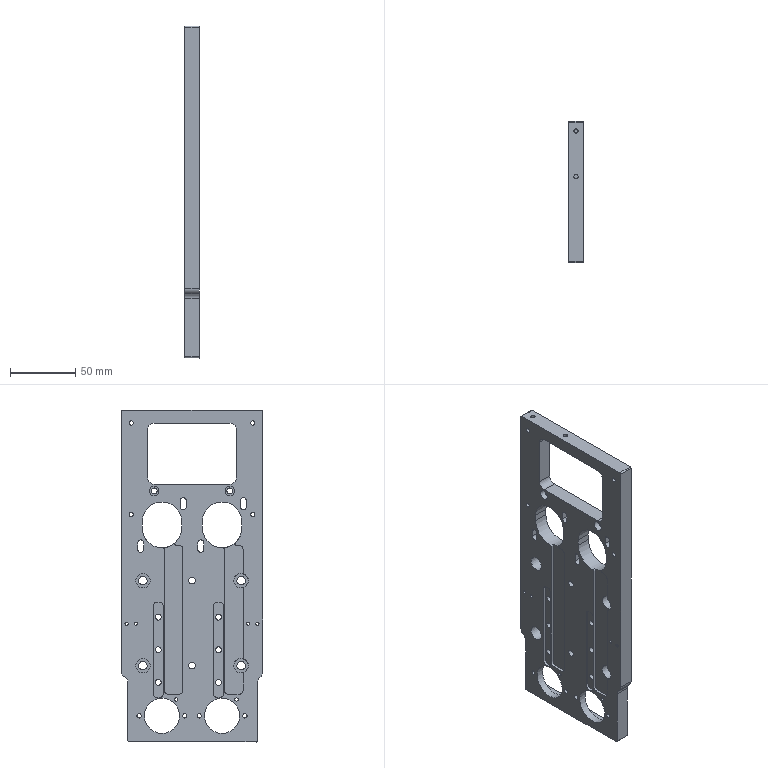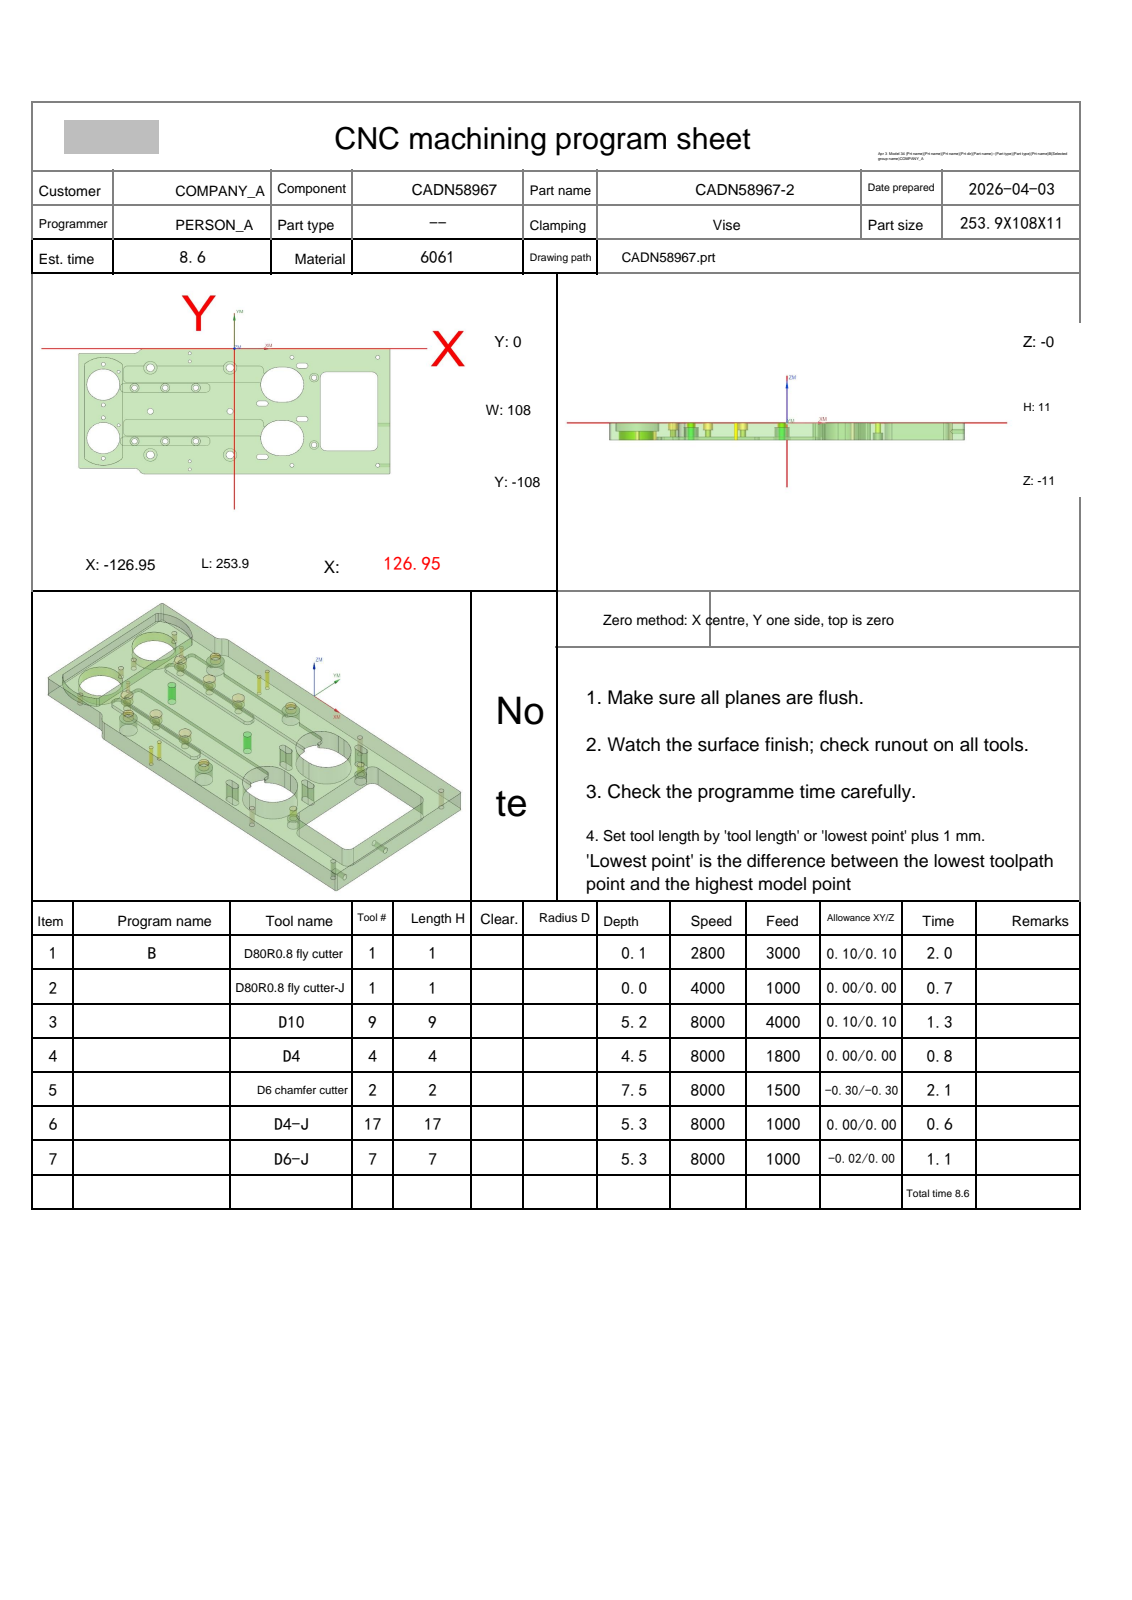NC program | NX | posted by the shop | part box 11 x 108 x 253.9 mm
Lines 1506 to 2432 of 3878:
N6 T17 M06
(D4-J  D=4. R=0. H=17 ce=0.00 di=0.00)
G00 G90 G54 X-118.616 Y-13.414 M03 S8000
G43 H17 Z20.
M08
Z.159
G01 X-118.62 Y-13.41 Z.098 F1000.
X-118.631 Y-13.401 Z.044
X-118.649 Y-13.386 Z-.005
X-118.673 Y-13.368 Z-.049
X-118.702 Y-13.347 Z-.087
X-118.736 Y-13.326 Z-.12
X-118.775 Y-13.305 Z-.148
X-118.817 Y-13.286 Z-.172
X-118.863 Y-13.269 Z-.192
X-118.911 Y-13.258 Z-.208
X-118.962 Y-13.252 Z-.221
X-119.014 Y-13.253 Z-.23
X-119.066 Y-13.262 Z-.236
X-119.12 Y-13.282 Z-.24
X-119.173 Y-13.312 Z-.241
G03 X-120.45 Y-14.267 I12.223 J-17.688
G01 Y-15.771
X-120.437 Y-15.822
X-120.399 Y-15.843 Z-.242
X-120.341 Y-15.837 Z-.244
X-120.265 Y-15.806 Z-.247
X-120.177 Y-15.754 Z-.251
X-120.078 Y-15.682 Z-.256
X-119.974 Y-15.594 Z-.262
X-119.868 Y-15.493 Z-.27
X-119.763 Y-15.38 Z-.279
X-119.546 Y-15.098 Z-.304
X-119.359 Y-14.785 Z-.335
X-119.21 Y-14.452 Z-.368
X-119.103 Y-14.11 Z-.401
X-119.071 Y-13.958 Z-.415
X-119.048 Y-13.812 Z-.429
X-119.035 Y-13.675 Z-.441
X-119.032 Y-13.552 Z-.453
X-119.039 Y-13.447 Z-.462
X-119.057 Y-13.367 Z-.471
X-119.085 Y-13.314 Z-.477
X-119.123 Y-13.294 Z-.48
X-119.173 Y-13.312 Z-.482
G03 X-120.45 Y-14.267 I12.223 J-17.688
G01 Y-15.771
X-120.437 Y-15.822
X-120.399 Y-15.844 Z-.483
X-120.341 Y-15.838 Z-.485
X-120.265 Y-15.808 Z-.488
X-120.177 Y-15.756 Z-.493
X-120.079 Y-15.686 Z-.498
X-119.974 Y-15.599 Z-.504
X-119.868 Y-15.498 Z-.512
X-119.763 Y-15.386 Z-.521
X-119.546 Y-15.104 Z-.546
X-119.359 Y-14.791 Z-.577
X-119.21 Y-14.457 Z-.61
X-119.103 Y-14.113 Z-.643
X-119.071 Y-13.961 Z-.657
X-119.048 Y-13.814 Z-.67
X-119.035 Y-13.676 Z-.683
X-119.032 Y-13.553 Z-.694
X-119.039 Y-13.448 Z-.704
X-119.057 Y-13.367 Z-.712
X-119.085 Y-13.314 Z-.718
X-119.123 Y-13.295 Z-.721
X-119.173 Y-13.312 Z-.723
G03 X-120.45 Y-14.267 I12.223 J-17.688
G01 Y-15.771
X-120.437 Y-15.823
X-120.399 Y-15.844 Z-.724
X-120.341 Y-15.839 Z-.727
X-120.265 Y-15.81 Z-.73
X-120.177 Y-15.759 Z-.734
X-120.079 Y-15.689 Z-.739
X-119.975 Y-15.603 Z-.746
X-119.868 Y-15.503 Z-.754
X-119.764 Y-15.392 Z-.763
X-119.587 Y-15.17 Z-.783
X-119.43 Y-14.925 Z-.806
X-119.295 Y-14.664 Z-.832
X-119.185 Y-14.393 Z-.858
X-119.104 Y-14.117 Z-.884
X-119.071 Y-13.964 Z-.898
X-119.048 Y-13.816 Z-.911
X-119.035 Y-13.678 Z-.924
X-119.032 Y-13.554 Z-.935
X-119.039 Y-13.449 Z-.945
X-119.057 Y-13.368 Z-.953
X-119.085 Y-13.315 Z-.959
X-119.123 Y-13.295 Z-.962
X-119.173 Y-13.312 Z-.964
G03 X-120.45 Y-14.267 I12.223 J-17.688
G01 Y-15.771
X-120.437 Y-15.823
X-120.399 Y-15.845 Z-.965
X-120.341 Y-15.841 Z-.968
X-120.265 Y-15.812 Z-.971
X-120.177 Y-15.762 Z-.975
X-120.079 Y-15.693 Z-.981
X-119.975 Y-15.608 Z-.988
X-119.869 Y-15.508 Z-.996
X-119.764 Y-15.397 Z-1.005
X-119.588 Y-15.176 Z-1.025
X-119.43 Y-14.931 Z-1.048
X-119.296 Y-14.67 Z-1.074
X-119.186 Y-14.397 Z-1.1
X-119.104 Y-14.12 Z-1.126
X-119.071 Y-13.966 Z-1.14
X-119.048 Y-13.818 Z-1.153
X-119.035 Y-13.679 Z-1.165
X-119.032 Y-13.555 Z-1.176
X-119.039 Y-13.45 Z-1.186
X-119.057 Y-13.368 Z-1.194
X-119.085 Y-13.315 Z-1.199
X-119.123 Y-13.295 Z-1.203
X-119.173 Y-13.312 Z-1.205
G03 X-120.45 Y-14.267 I12.223 J-17.688
G01 Y-15.771
X-120.437 Y-15.823
X-120.399 Y-15.846 Z-1.206
X-120.341 Y-15.842 Z-1.209
X-120.266 Y-15.814 Z-1.212
X-120.177 Y-15.765 Z-1.217
X-120.079 Y-15.697 Z-1.223
X-119.975 Y-15.612 Z-1.229
X-119.869 Y-15.514 Z-1.238
X-119.765 Y-15.403 Z-1.247
X-119.588 Y-15.182 Z-1.267
X-119.431 Y-14.937 Z-1.29
X-119.296 Y-14.675 Z-1.315
X-119.186 Y-14.401 Z-1.342
X-119.104 Y-14.123 Z-1.367
X-119.072 Y-13.969 Z-1.381
X-119.049 Y-13.82 Z-1.394
X-119.035 Y-13.681 Z-1.406
X-119.032 Y-13.556 Z-1.417
X-119.039 Y-13.451 Z-1.427
X-119.057 Y-13.369 Z-1.435
X-119.085 Y-13.315 Z-1.44
X-119.123 Y-13.295 Z-1.444
X-119.173 Y-13.312 Z-1.445
G03 X-120.45 Y-14.267 I12.223 J-17.688
G01 Y-15.771
X-120.437 Y-15.823 Z-1.446
X-120.399 Y-15.846 Z-1.447
X-120.341 Y-15.843 Z-1.45
X-120.266 Y-15.816 Z-1.454
X-120.178 Y-15.768 Z-1.458
X-120.08 Y-15.701 Z-1.464
X-119.976 Y-15.617 Z-1.471
X-119.87 Y-15.519 Z-1.48
X-119.765 Y-15.409 Z-1.489
X-119.589 Y-15.188 Z-1.509
X-119.432 Y-14.943 Z-1.532
X-119.297 Y-14.68 Z-1.557
X-119.187 Y-14.406 Z-1.583
X-119.105 Y-14.126 Z-1.609
X-119.072 Y-13.972 Z-1.623
X-119.049 Y-13.822 Z-1.635
X-119.036 Y-13.683 Z-1.648
X-119.033 Y-13.557 Z-1.658
X-119.039 Y-13.451 Z-1.668
X-119.057 Y-13.369 Z-1.676
X-119.085 Y-13.315 Z-1.681
X-119.123 Y-13.295 Z-1.685
X-119.173 Y-13.312 Z-1.686
G03 X-120.45 Y-14.267 I12.223 J-17.688
G01 Y-15.771
X-120.437 Y-15.823 Z-1.687
X-120.399 Y-15.847 Z-1.688
X-120.341 Y-15.844 Z-1.691
X-120.266 Y-15.818 Z-1.695
X-120.178 Y-15.771 Z-1.7
X-120.08 Y-15.704 Z-1.706
X-119.977 Y-15.621 Z-1.713
X-119.871 Y-15.524 Z-1.722
X-119.766 Y-15.415 Z-1.731
X-119.59 Y-15.194 Z-1.751
X-119.433 Y-14.949 Z-1.774
X-119.298 Y-14.685 Z-1.799
X-119.187 Y-14.41 Z-1.825
X-119.105 Y-14.13 Z-1.85
X-119.072 Y-13.975 Z-1.864
X-119.049 Y-13.825 Z-1.877
X-119.036 Y-13.684 Z-1.889
X-119.033 Y-13.559 Z-1.9
X-119.04 Y-13.452 Z-1.909
X-119.057 Y-13.369 Z-1.917
X-119.085 Y-13.316 Z-1.922
X-119.123 Y-13.295 Z-1.926
X-119.173 Y-13.312 Z-1.927
G03 X-120.45 Y-14.267 I12.223 J-17.688
G01 Y-15.771
X-120.437 Y-15.823 Z-1.928
X-120.399 Y-15.847 Z-1.93
X-120.341 Y-15.845 Z-1.932
X-120.267 Y-15.82 Z-1.936
X-120.179 Y-15.774 Z-1.941
X-120.081 Y-15.708 Z-1.948
X-119.978 Y-15.626 Z-1.955
X-119.872 Y-15.529 Z-1.964
X-119.767 Y-15.421 Z-1.973
X-119.591 Y-15.201 Z-1.994
X-119.434 Y-14.955 Z-2.017
X-119.299 Y-14.691 Z-2.041
X-119.188 Y-14.415 Z-2.067
X-119.106 Y-14.133 Z-2.092
X-119.073 Y-13.977 Z-2.105
X-119.05 Y-13.827 Z-2.118
X-119.036 Y-13.686 Z-2.13
X-119.033 Y-13.56 Z-2.141
X-119.04 Y-13.453 Z-2.15
X-119.057 Y-13.37 Z-2.158
X-119.085 Y-13.316 Z-2.163
X-119.123 Y-13.295 Z-2.167
X-119.173 Y-13.312 Z-2.168
G03 X-120.45 Y-14.267 I12.223 J-17.688
G01 Y-15.771
X-120.437 Y-15.824 Z-2.169
X-120.399 Y-15.848 Z-2.171
X-120.342 Y-15.847 Z-2.173
X-120.267 Y-15.822 Z-2.178
X-120.179 Y-15.776 Z-2.183
X-120.082 Y-15.712 Z-2.189
X-119.979 Y-15.631 Z-2.197
X-119.873 Y-15.535 Z-2.206
X-119.769 Y-15.427 Z-2.215
X-119.593 Y-15.207 Z-2.236
X-119.435 Y-14.961 Z-2.259
X-119.3 Y-14.696 Z-2.284
X-119.189 Y-14.419 Z-2.309
X-119.106 Y-14.136 Z-2.334
X-119.073 Y-13.98 Z-2.347
X-119.05 Y-13.829 Z-2.36
X-119.037 Y-13.688 Z-2.371
X-119.033 Y-13.561 Z-2.382
X-119.04 Y-13.454 Z-2.391
X-119.057 Y-13.37 Z-2.399
X-119.085 Y-13.316 Z-2.404
X-119.123 Y-13.295 Z-2.408
X-119.173 Y-13.312 Z-2.409
G03 X-120.45 Y-14.267 I12.223 J-17.688
G01 Y-15.771
X-120.437 Y-15.824 Z-2.41
X-120.4 Y-15.848 Z-2.412
X-120.342 Z-2.415
X-120.268 Y-15.824 Z-2.419
X-120.18 Y-15.779 Z-2.424
X-120.083 Y-15.716 Z-2.431
X-119.98 Y-15.635 Z-2.439
X-119.874 Y-15.54 Z-2.448
X-119.77 Y-15.432 Z-2.458
X-119.594 Y-15.213 Z-2.478
X-119.437 Y-14.967 Z-2.501
X-119.301 Y-14.701 Z-2.526
X-119.19 Y-14.423 Z-2.551
X-119.107 Y-14.14 Z-2.575
X-119.074 Y-13.983 Z-2.588
X-119.051 Y-13.831 Z-2.601
X-119.037 Y-13.689 Z-2.613
X-119.034 Y-13.562 Z-2.623
X-119.04 Y-13.454 Z-2.632
X-119.057 Y-13.371 Z-2.64
X-119.085 Y-13.316 Z-2.645
X-119.123 Y-13.295 Z-2.649
X-119.173 Y-13.312 Z-2.65
G03 X-120.45 Y-14.267 I12.223 J-17.688
G01 Y-15.771
X-120.437 Y-15.824 Z-2.651
X-120.4 Y-15.849 Z-2.653
X-120.342 Z-2.656
X-120.268 Y-15.826 Z-2.66
X-120.181 Y-15.782 Z-2.666
X-120.084 Y-15.719 Z-2.673
X-119.981 Y-15.64 Z-2.681
X-119.876 Y-15.545 Z-2.69
X-119.772 Y-15.438 Z-2.7
X-119.596 Y-15.219 Z-2.72
X-119.439 Y-14.973 Z-2.743
X-119.303 Y-14.707 Z-2.768
X-119.192 Y-14.428 Z-2.793
X-119.108 Y-14.143 Z-2.817
X-119.078 Y-14.001 Z-2.829
X-119.055 Y-13.863 Z-2.84
X-119.041 Y-13.732 Z-2.85
X-119.034 Y-13.612 Z-2.86
X-119.036 Y-13.507 Z-2.869
X-119.046 Y-13.419 Z-2.876
X-119.064 Y-13.352 Z-2.882
X-119.092 Y-13.309 Z-2.887
X-119.128 Y-13.295 Z-2.89
X-119.173 Y-13.312 Z-2.891
G03 X-120.45 Y-14.267 I12.223 J-17.688
G01 Y-15.771
X-120.437 Y-15.824 Z-2.892
X-120.4 Y-15.85 Z-2.894
X-120.343 Z-2.897
X-120.269 Y-15.828 Z-2.902
X-120.182 Y-15.785 Z-2.908
X-120.085 Y-15.723 Z-2.915
X-119.983 Y-15.644 Z-2.923
X-119.878 Y-15.55 Z-2.932
X-119.774 Y-15.444 Z-2.942
X-119.598 Y-15.225 Z-2.963
X-119.441 Y-14.979 Z-2.986
X-119.305 Y-14.712 Z-3.01
X-119.193 Y-14.432 Z-3.034
X-119.109 Y-14.146 Z-3.059
X-119.079 Y-14.004 Z-3.07
X-119.056 Y-13.865 Z-3.081
X-119.041 Y-13.734 Z-3.092
X-119.035 Y-13.614 Z-3.101
X-119.036 Y-13.508 Z-3.11
X-119.046 Y-13.419 Z-3.117
X-119.065 Y-13.352 Z-3.123
X-119.092 Y-13.309 Z-3.128
X-119.128 Y-13.295 Z-3.131
X-119.173 Y-13.312 Z-3.132
G03 X-120.45 Y-14.267 I12.223 J-17.688
G01 Y-15.771
X-120.437 Y-15.824 Z-3.133
X-120.4 Y-15.85 Z-3.135
X-120.343 Y-15.852 Z-3.138
X-120.27 Y-15.83 Z-3.143
X-120.183 Y-15.788 Z-3.149
X-120.087 Y-15.727 Z-3.156
X-119.984 Y-15.649 Z-3.165
X-119.88 Y-15.556 Z-3.174
X-119.776 Y-15.45 Z-3.184
X-119.6 Y-15.231 Z-3.205
X-119.443 Y-14.985 Z-3.228
X-119.307 Y-14.717 Z-3.252
X-119.195 Y-14.436 Z-3.276
X-119.111 Y-14.149 Z-3.3
X-119.08 Y-14.006 Z-3.312
X-119.057 Y-13.867 Z-3.323
X-119.042 Y-13.736 Z-3.333
X-119.035 Y-13.615 Z-3.343
X-119.037 Y-13.509 Z-3.351
X-119.046 Y-13.42 Z-3.358
X-119.065 Y-13.352 Z-3.364
X-119.092 Y-13.31 Z-3.369
X-119.128 Y-13.295 Z-3.372
X-119.173 Y-13.312 Z-3.373
G03 X-120.45 Y-14.267 I12.223 J-17.688
G01 Y-15.771
X-120.437 Y-15.824 Z-3.374
X-120.4 Y-15.851 Z-3.376
X-120.344 Y-15.853 Z-3.379
X-120.27 Y-15.832 Z-3.384
X-120.184 Y-15.791 Z-3.391
X-120.088 Y-15.73 Z-3.398
X-119.986 Y-15.653 Z-3.407
X-119.882 Y-15.561 Z-3.416
X-119.778 Y-15.455 Z-3.427
X-119.603 Y-15.237 Z-3.447
X-119.445 Y-14.99 Z-3.47
X-119.309 Y-14.722 Z-3.494
X-119.196 Y-14.44 Z-3.518
X-119.112 Y-14.152 Z-3.542
X-119.081 Y-14.009 Z-3.553
X-119.058 Y-13.87 Z-3.564
X-119.043 Y-13.738 Z-3.574
X-119.036 Y-13.616 Z-3.584
X-119.037 Y-13.509 Z-3.592
X-119.047 Y-13.42 Z-3.6
X-119.065 Y-13.353 Z-3.605
X-119.092 Y-13.31 Z-3.61
X-119.128 Y-13.295 Z-3.613
X-119.173 Y-13.312 Z-3.614
G03 X-120.45 Y-14.267 I12.223 J-17.688
G01 Y-15.771
X-120.437 Y-15.824
X-120.401 Y-15.851 Z-3.617
X-120.344 Y-15.854 Z-3.621
X-120.271 Y-15.834 Z-3.626
X-120.185 Y-15.793 Z-3.632
X-120.09 Y-15.734 Z-3.64
X-119.988 Y-15.657 Z-3.649
X-119.884 Y-15.566 Z-3.658
X-119.781 Y-15.461 Z-3.669
X-119.605 Y-15.243 Z-3.69
X-119.448 Y-14.996 Z-3.713
X-119.311 Y-14.727 Z-3.736
X-119.198 Y-14.445 Z-3.76
X-119.113 Y-14.156 Z-3.784
X-119.082 Y-14.012 Z-3.795
X-119.059 Y-13.872 Z-3.806
X-119.043 Y-13.739 Z-3.816
X-119.036 Y-13.618 Z-3.825
X-119.037 Y-13.51 Z-3.833
X-119.047 Y-13.421 Z-3.841
X-119.065 Y-13.353 Z-3.846
X-119.092 Y-13.31 Z-3.851
X-119.128 Y-13.295 Z-3.854
X-119.173 Y-13.312 Z-3.855
G03 X-120.45 Y-14.267 I12.223 J-17.688
G01 Y-15.771
X-120.437 Y-15.825
X-120.401 Y-15.852 Z-3.858
X-120.345 Y-15.855 Z-3.862
X-120.272 Y-15.836 Z-3.867
X-120.187 Y-15.796 Z-3.874
X-120.092 Y-15.737 Z-3.882
X-119.99 Y-15.662 Z-3.891
X-119.886 Y-15.571 Z-3.9
X-119.783 Y-15.466 Z-3.911
X-119.608 Y-15.249 Z-3.932
X-119.451 Y-15.002 Z-3.955
X-119.313 Y-14.732 Z-3.978
X-119.2 Y-14.449 Z-4.002
X-119.115 Y-14.159 Z-4.025
X-119.083 Y-14.014 Z-4.036
X-119.06 Y-13.874 Z-4.047
X-119.044 Y-13.741 Z-4.057
X-119.037 Y-13.619 Z-4.066
X-119.038 Y-13.511 Z-4.075
X-119.047 Y-13.422 Z-4.082
X-119.065 Y-13.353 Z-4.087
X-119.092 Y-13.31 Z-4.092
X-119.128 Y-13.295 Z-4.095
X-119.173 Y-13.312
G03 X-120.45 Y-14.267 I12.223 J-17.688
G01 Y-15.771
X-120.437 Y-15.825 Z-4.096
X-120.401 Y-15.852 Z-4.099
X-120.345 Y-15.856 Z-4.103
X-120.273 Y-15.838 Z-4.109
X-120.188 Y-15.799 Z-4.115
X-120.093 Y-15.741 Z-4.124
X-119.993 Y-15.666 Z-4.133
X-119.889 Y-15.576 Z-4.143
X-119.786 Y-15.472 Z-4.154
X-119.611 Y-15.255 Z-4.175
X-119.453 Y-15.007 Z-4.197
X-119.316 Y-14.737 Z-4.221
X-119.203 Y-14.453 Z-4.244
X-119.116 Y-14.162 Z-4.267
X-119.085 Y-14.017 Z-4.278
X-119.061 Y-13.876 Z-4.289
X-119.045 Y-13.743 Z-4.298
X-119.038 Y-13.62 Z-4.308
Y-13.512 Z-4.316
X-119.048 Y-13.422 Z-4.323
X-119.065 Y-13.354 Z-4.328
X-119.092 Y-13.31 Z-4.333
X-119.128 Y-13.295 Z-4.335
X-119.173 Y-13.312 Z-4.336
G03 X-120.45 Y-14.267 I12.223 J-17.688
G01 Y-15.771
X-120.435 Y-15.831 Z-4.338
X-120.394 Y-15.862 Z-4.342
X-120.331 Y-15.865 Z-4.348
X-120.25 Y-15.843 Z-4.356
X-120.155 Y-15.795 Z-4.366
X-120.051 Y-15.726 Z-4.377
X-119.941 Y-15.635 Z-4.389
X-119.83 Y-15.524 Z-4.402
X-119.658 Y-15.311 Z-4.423
X-119.498 Y-15.061 Z-4.446
X-119.356 Y-14.785 Z-4.468
X-119.235 Y-14.492 Z-4.49
X-119.141 Y-14.191 Z-4.512
X-119.105 Y-14.042 Z-4.522
X-119.078 Y-13.896 Z-4.532
X-119.059 Y-13.759 Z-4.542
X-119.048 Y-13.632 Z-4.55
X-119.046 Y-13.521 Z-4.558
X-119.052 Y-13.428 Z-4.564
X-119.068 Y-13.357 Z-4.57
X-119.093 Y-13.312 Z-4.574
X-119.128 Y-13.296 Z-4.576
X-119.173 Y-13.312 Z-4.577
G03 X-120.45 Y-14.267 I12.223 J-17.688
G01 Y-15.771
X-120.435 Y-15.831 Z-4.579
X-120.394 Y-15.862 Z-4.583
X-120.331 Y-15.865 Z-4.589
X-120.25 Y-15.843 Z-4.597
X-120.155 Y-15.795 Z-4.606
X-120.051 Y-15.726 Z-4.618
X-119.941 Y-15.635 Z-4.63
X-119.83 Y-15.524 Z-4.643
X-119.658 Y-15.311 Z-4.664
X-119.498 Y-15.061 Z-4.686
X-119.356 Y-14.785 Z-4.709
X-119.235 Y-14.492 Z-4.731
X-119.141 Y-14.191 Z-4.753
X-119.105 Y-14.042 Z-4.763
X-119.078 Y-13.896 Z-4.773
X-119.059 Y-13.759 Z-4.783
X-119.048 Y-13.632 Z-4.791
X-119.046 Y-13.521 Z-4.799
X-119.052 Y-13.428 Z-4.805
X-119.068 Y-13.357 Z-4.811
X-119.093 Y-13.312 Z-4.815
X-119.128 Y-13.296 Z-4.817
X-119.173 Y-13.312 Z-4.818
G03 X-120.45 Y-14.267 I12.223 J-17.688
G01 Y-15.771
X-120.435 Y-15.831 Z-4.82
X-120.394 Y-15.862 Z-4.823
X-120.331 Y-15.865 Z-4.83
X-120.25 Y-15.843 Z-4.838
X-120.155 Y-15.795 Z-4.847
X-120.051 Y-15.726 Z-4.858
X-119.941 Y-15.635 Z-4.871
X-119.83 Y-15.524 Z-4.883
X-119.658 Y-15.311 Z-4.905
X-119.498 Y-15.061 Z-4.927
X-119.356 Y-14.785 Z-4.95
X-119.235 Y-14.492 Z-4.972
X-119.141 Y-14.191 Z-4.994
X-119.105 Y-14.042 Z-5.004
X-119.078 Y-13.896 Z-5.014
X-119.059 Y-13.759 Z-5.023
X-119.048 Y-13.632 Z-5.032
X-119.046 Y-13.521 Z-5.04
X-119.052 Y-13.428 Z-5.046
X-119.068 Y-13.357 Z-5.052
X-119.093 Y-13.312 Z-5.056
X-119.128 Y-13.296 Z-5.058
X-119.173 Y-13.312 Z-5.059
G03 X-120.45 Y-14.267 I12.223 J-17.688
G01 Y-15.771
X-120.435 Y-15.831 Z-5.06
X-120.394 Y-15.862 Z-5.064
X-120.331 Y-15.865 Z-5.07
X-120.25 Y-15.843 Z-5.079
X-120.155 Y-15.795 Z-5.088
X-120.051 Y-15.726 Z-5.099
X-119.941 Y-15.635 Z-5.111
X-119.83 Y-15.524 Z-5.124
X-119.658 Y-15.311 Z-5.146
X-119.498 Y-15.061 Z-5.168
X-119.356 Y-14.785 Z-5.191
X-119.235 Y-14.492 Z-5.213
X-119.141 Y-14.191 Z-5.235
X-119.105 Y-14.042 Z-5.245
X-119.078 Y-13.896 Z-5.255
X-119.059 Y-13.759 Z-5.264
X-119.048 Y-13.632 Z-5.273
X-119.046 Y-13.521 Z-5.281
X-119.052 Y-13.428 Z-5.287
X-119.068 Y-13.357 Z-5.293
X-119.093 Y-13.312 Z-5.297
X-119.128 Y-13.296 Z-5.299
X-119.173 Y-13.312 Z-5.3
G03 X-120.45 Y-14.267 I12.223 J-17.688
G01 Y-15.771
X-120.419 Y-15.835 Z-5.299
X-120.384 Y-15.9 Z-5.295
X-120.346 Y-15.966 Z-5.287
X-120.306 Y-16.032 Z-5.277
X-120.266 Y-16.096 Z-5.262
X-120.225 Y-16.159 Z-5.243
X-120.186 Y-16.217 Z-5.22
X-120.149 Y-16.272 Z-5.192
X-120.114 Y-16.32 Z-5.158
X-120.084 Y-16.363 Z-5.119
X-120.059 Y-16.397 Z-5.074
X-120.04 Y-16.423 Z-5.023
X-120.028 Y-16.44 Z-4.965
X-120.023 Y-16.445 Z-4.9
G00 Z3.
X-120.049 Y-91.829
Z.159
G01 X-120.054 Y-91.83 Z.098
X-120.068 Y-91.833 Z.044
X-120.091 Y-91.839 Z-.005
X-120.119 Y-91.849 Z-.049
X-120.153 Y-91.861 Z-.087
X-120.19 Y-91.877 Z-.12
X-120.229 Y-91.897 Z-.148
X-120.269 Y-91.921 Z-.172
X-120.309 Y-91.949 Z-.192
X-120.346 Y-91.983 Z-.208
X-120.38 Y-92.021 Z-.221
X-120.408 Y-92.064 Z-.23
X-120.431 Y-92.113 Z-.236
X-120.445 Y-92.168 Z-.24
X-120.45 Y-92.229 Z-.241
Y-93.724
Y-93.733
G03 X-119.173 Y-94.688 I13.5 J16.733
G01 X-119.123 Y-94.706 Z-.242
X-119.083 Y-94.687 Z-.245
X-119.052 Y-94.637 Z-.25
X-119.032 Y-94.558 Z-.257
X-119.022 Y-94.456 Z-.264
Y-94.336 Z-.274
X-119.032 Y-94.201 Z-.284
X-119.052 Y-94.057 Z-.295
X-119.083 Y-93.907 Z-.306
X-119.163 Y-93.635 Z-.328
X-119.273 Y-93.365 Z-.35
X-119.41 Y-93.105 Z-.373
X-119.57 Y-92.859 Z-.395
X-119.75 Y-92.633 Z-.416
X-119.857 Y-92.519 Z-.428
X-119.966 Y-92.415 Z-.439
X-120.072 Y-92.325 Z-.449
X-120.172 Y-92.252 Z-.458
X-120.262 Y-92.198 Z-.466
X-120.339 Y-92.165 Z-.473
X-120.398 Y-92.158 Z-.478
X-120.436 Y-92.178 Z-.481
X-120.45 Y-92.229 Z-.482
Y-93.724
Y-93.733
G03 X-119.173 Y-94.688 I13.5 J16.733
G01 X-119.122 Y-94.706
X-119.082 Y-94.688 Z-.484
X-119.052 Y-94.637 Z-.486
X-119.031 Y-94.559 Z-.49
X-119.02 Y-94.458 Z-.494
Y-94.338 Z-.5
X-119.029 Y-94.204 Z-.507
X-119.049 Y-94.06 Z-.515
X-119.079 Y-93.911 Z-.524
X-119.159 Y-93.639 Z-.544
X-119.27 Y-93.369 Z-.567
X-119.407 Y-93.108 Z-.593
X-119.568 Y-92.862 Z-.619
X-119.748 Y-92.635 Z-.644
X-119.856 Y-92.521 Z-.658
X-119.964 Y-92.417 Z-.671
X-120.071 Y-92.327 Z-.683
X-120.171 Y-92.253 Z-.694
X-120.261 Y-92.198 Z-.704
X-120.338 Y-92.166 Z-.712
X-120.398 Y-92.158 Z-.718
X-120.436 Y-92.178 Z-.721
X-120.45 Y-92.229 Z-.723
Y-93.724
Y-93.733
G03 X-119.173 Y-94.688 I13.5 J16.733
G01 X-119.122 Y-94.706
X-119.082 Y-94.688 Z-.725
X-119.051 Y-94.638 Z-.727
X-119.03 Y-94.561 Z-.731
X-119.019 Y-94.46 Z-.735
X-119.017 Y-94.34 Z-.741
X-119.026 Y-94.207 Z-.748
X-119.046 Y-94.063 Z-.757
X-119.076 Y-93.914 Z-.766
X-119.155 Y-93.642 Z-.786
X-119.266 Y-93.373 Z-.809
X-119.403 Y-93.111 Z-.834
X-119.565 Y-92.864 Z-.86
X-119.746 Y-92.637 Z-.886
X-119.854 Y-92.522 Z-.9
X-119.963 Y-92.418 Z-.913
X-120.07 Y-92.327 Z-.925
X-120.17 Y-92.253 Z-.936
X-120.261 Y-92.199 Z-.945
X-120.338 Y-92.166 Z-.953
X-120.398 Y-92.158 Z-.959
X-120.436 Y-92.178 Z-.962
X-120.45 Y-92.229 Z-.964
Y-93.724
Y-93.733
G03 X-119.173 Y-94.688 I13.5 J16.733
G01 X-119.122 Y-94.706
X-119.081 Y-94.688 Z-.966
X-119.05 Y-94.639 Z-.968
X-119.028 Y-94.562 Z-.972
X-119.017 Y-94.462 Z-.977
X-119.015 Y-94.343 Z-.983
X-119.024 Y-94.209 Z-.99
X-119.042 Y-94.066 Z-.998
X-119.072 Y-93.917 Z-1.008
X-119.151 Y-93.646 Z-1.028
X-119.262 Y-93.376 Z-1.051
X-119.4 Y-93.114 Z-1.076
X-119.562 Y-92.867 Z-1.102
X-119.744 Y-92.639 Z-1.127
X-119.852 Y-92.524 Z-1.141
X-119.961 Y-92.419 Z-1.154
X-120.069 Y-92.328 Z-1.166
X-120.169 Y-92.254 Z-1.177
X-120.26 Y-92.199 Z-1.186
X-120.338 Y-92.166 Z-1.194
X-120.398 Y-92.158 Z-1.2
X-120.436 Y-92.178 Z-1.203
X-120.45 Y-92.229 Z-1.205
Y-93.724
Y-93.733
G03 X-119.173 Y-94.688 I13.5 J16.733
G01 X-119.122 Y-94.706
X-119.081 Y-94.689 Z-1.207
X-119.049 Y-94.639 Z-1.209
X-119.027 Y-94.563 Z-1.213
X-119.015 Y-94.463 Z-1.218
X-119.013 Y-94.345 Z-1.224
X-119.021 Y-94.212 Z-1.232
X-119.039 Y-94.069 Z-1.24
X-119.068 Y-93.921 Z-1.25
X-119.147 Y-93.649 Z-1.27
X-119.258 Y-93.38 Z-1.293
X-119.396 Y-93.118 Z-1.318
X-119.559 Y-92.869 Z-1.344
X-119.742 Y-92.641 Z-1.369
X-119.85 Y-92.525 Z-1.382
X-119.96 Y-92.421 Z-1.395
X-120.067 Y-92.329 Z-1.407
X-120.169 Y-92.255 Z-1.418
X-120.26 Y-92.2 Z-1.427
X-120.337 Y-92.166 Z-1.435
X-120.397 Y-92.158 Z-1.441
X-120.436 Y-92.178 Z-1.444
X-120.45 Y-92.229 Z-1.445
Y-93.724
Y-93.733
G03 X-119.173 Y-94.688 I13.5 J16.733
G01 X-119.122 Y-94.706 Z-1.446
X-119.081 Y-94.689 Z-1.448
X-119.049 Y-94.64 Z-1.451
X-119.026 Y-94.564 Z-1.455
X-119.013 Y-94.465 Z-1.46
X-119.01 Y-94.347 Z-1.466
X-119.018 Y-94.215 Z-1.473
X-119.036 Y-94.073 Z-1.482
X-119.065 Y-93.924 Z-1.492
X-119.143 Y-93.653 Z-1.512
X-119.254 Y-93.383 Z-1.535
X-119.393 Y-93.121 Z-1.56
X-119.556 Y-92.872 Z-1.585
X-119.74 Y-92.643 Z-1.61
X-119.849 Y-92.527 Z-1.624
X-119.959 Y-92.422 Z-1.636
X-120.066 Y-92.33 Z-1.648
X-120.168 Y-92.256 Z-1.659
X-120.259 Y-92.2 Z-1.668
X-120.337 Y-92.167 Z-1.676
X-120.397 Y-92.159 Z-1.681
X-120.436 Y-92.178 Z-1.685
X-120.45 Y-92.229 Z-1.686
Y-93.724
Y-93.733
G03 X-119.173 Y-94.688 I13.5 J16.733
G01 X-119.122 Y-94.706 Z-1.687
X-119.08 Y-94.689 Z-1.689
X-119.048 Y-94.641 Z-1.692
X-119.025 Y-94.565 Z-1.696
X-119.011 Y-94.467 Z-1.701
X-119.008 Y-94.35 Z-1.708
X-119.015 Y-94.218 Z-1.715
X-119.033 Y-94.076 Z-1.724
X-119.061 Y-93.928 Z-1.734
X-119.14 Y-93.657 Z-1.754
X-119.251 Y-93.387 Z-1.777
X-119.39 Y-93.124 Z-1.802
X-119.554 Y-92.875 Z-1.827
X-119.738 Y-92.645 Z-1.852
X-119.847 Y-92.529 Z-1.865
X-119.957 Y-92.423 Z-1.878
X-120.065 Y-92.332 Z-1.889
X-120.167 Y-92.256 Z-1.9
X-120.259 Y-92.201 Z-1.909
X-120.337 Y-92.167 Z-1.917
X-120.397 Y-92.159 Z-1.922
X-120.436 Y-92.178 Z-1.926
X-120.45 Y-92.229 Z-1.927
Y-93.724
Y-93.733
G03 X-119.173 Y-94.688 I13.5 J16.733
G01 X-119.122 Y-94.707 Z-1.928
X-119.08 Y-94.69 Z-1.93
X-119.047 Y-94.642 Z-1.933
X-119.024 Y-94.567 Z-1.937
X-119.01 Y-94.469 Z-1.943
X-119.006 Y-94.352 Z-1.949
X-119.012 Y-94.221 Z-1.957
X-119.029 Y-94.079 Z-1.966
X-119.058 Y-93.932 Z-1.976
X-119.136 Y-93.661 Z-1.996
X-119.247 Y-93.391 Z-2.019
X-119.387 Y-93.128 Z-2.044
X-119.551 Y-92.878 Z-2.069
X-119.736 Y-92.647 Z-2.093
X-119.845 Y-92.531 Z-2.107
X-119.956 Y-92.425 Z-2.119
X-120.064 Y-92.333 Z-2.131
X-120.166 Y-92.257 Z-2.141
X-120.258 Y-92.201 Z-2.15
X-120.337 Y-92.167 Z-2.158
X-120.397 Y-92.159 Z-2.163
X-120.436 Y-92.178 Z-2.167
X-120.45 Y-92.229 Z-2.168
Y-93.724
Y-93.733
G03 X-119.173 Y-94.688 I13.5 J16.733
G01 X-119.122 Y-94.707 Z-2.169
X-119.08 Y-94.69 Z-2.171
X-119.046 Y-94.643 Z-2.174
X-119.022 Y-94.568 Z-2.178
X-119.008 Y-94.471 Z-2.184
X-119.004 Y-94.354 Z-2.191
X-119.01 Y-94.224 Z-2.199
X-119.026 Y-94.083 Z-2.208
X-119.054 Y-93.936 Z-2.218
X-119.132 Y-93.665 Z-2.238
X-119.244 Y-93.395 Z-2.261
X-119.384 Y-93.131 Z-2.286
X-119.548 Y-92.881 Z-2.311
X-119.734 Y-92.65 Z-2.335
X-119.832 Y-92.544 Z-2.347
X-119.933 Y-92.446 Z-2.358
X-120.031 Y-92.36 Z-2.369
X-120.126 Y-92.286 Z-2.378
X-120.213 Y-92.227 Z-2.387
X-120.291 Y-92.185 Z-2.394
X-120.356 Y-92.162 Z-2.401
X-120.407 Y-92.16 Z-2.405
X-120.439 Y-92.182 Z-2.408
X-120.45 Y-92.229 Z-2.409
Y-93.724
Y-93.733
G03 X-119.173 Y-94.688 I13.5 J16.733
G01 X-119.123 Y-94.706 Z-2.41
X-119.084 Y-94.686 Z-2.413
X-119.056 Y-94.634 Z-2.418
X-119.039 Y-94.553 Z-2.425
X-119.032 Y-94.45 Z-2.433
X-119.034 Y-94.327 Z-2.442
X-119.047 Y-94.191 Z-2.452
X-119.07 Y-94.044 Z-2.463
X-119.102 Y-93.893 Z-2.474
X-119.208 Y-93.552 Z-2.501
X-119.357 Y-93.221 Z-2.529
X-119.543 Y-92.908 Z-2.558
X-119.761 Y-92.626 Z-2.585
X-119.866 Y-92.513 Z-2.596
X-119.972 Y-92.411 Z-2.607
X-120.077 Y-92.322 Z-2.617
X-120.175 Y-92.249 Z-2.626
X-120.264 Y-92.196 Z-2.634
X-120.34 Y-92.164 Z-2.641
X-120.399 Y-92.157 Z-2.646
X-120.437 Y-92.178 Z-2.649
X-120.45 Y-92.229 Z-2.65
Y-93.724
Y-93.733
G03 X-119.173 Y-94.688 I13.5 J16.733
G01 X-119.123 Y-94.706 Z-2.651
X-119.084 Y-94.686 Z-2.654
X-119.056 Y-94.634 Z-2.659
X-119.039 Y-94.553 Z-2.666
X-119.032 Y-94.45 Z-2.674
X-119.034 Y-94.327 Z-2.683
X-119.047 Y-94.191 Z-2.693
X-119.07 Y-94.044 Z-2.704
X-119.102 Y-93.893 Z-2.715
X-119.208 Y-93.553 Z-2.742
X-119.357 Y-93.221 Z-2.77
X-119.543 Y-92.908 Z-2.798
X-119.76 Y-92.626 Z-2.826
X-119.866 Y-92.513 Z-2.837
X-119.972 Y-92.411 Z-2.848
X-120.077 Y-92.322 Z-2.858
X-120.175 Y-92.249 Z-2.867
X-120.264 Y-92.196 Z-2.875
X-120.34 Y-92.164 Z-2.882
X-120.399 Y-92.157 Z-2.887
X-120.437 Y-92.178 Z-2.89
X-120.45 Y-92.229 Z-2.891
Y-93.724
Y-93.733
G03 X-119.173 Y-94.688 I13.5 J16.733
G01 X-119.123 Y-94.706 Z-2.892
X-119.084 Y-94.686 Z-2.895
X-119.056 Y-94.634 Z-2.9
X-119.039 Y-94.553 Z-2.907
X-119.031 Y-94.45 Z-2.914
X-119.034 Y-94.327 Z-2.924
X-119.047 Y-94.191 Z-2.934
X-119.07 Y-94.044 Z-2.945
X-119.102 Y-93.893 Z-2.956
X-119.208 Y-93.553 Z-2.983
X-119.357 Y-93.221 Z-3.011
X-119.542 Y-92.908 Z-3.039
X-119.76 Y-92.626 Z-3.066
X-119.865 Y-92.513 Z-3.078
X-119.972 Y-92.411 Z-3.089
X-120.077 Y-92.322 Z-3.099
X-120.175 Y-92.249 Z-3.108
X-120.264 Y-92.196 Z-3.116
X-120.34 Y-92.164 Z-3.123
X-120.399 Y-92.157 Z-3.128
X-120.437 Y-92.178 Z-3.131
X-120.45 Y-92.229 Z-3.132
Y-93.724
Y-93.733
G03 X-119.173 Y-94.688 I13.5 J16.733
G01 X-119.123 Y-94.706 Z-3.133
X-119.084 Y-94.686 Z-3.136
X-119.056 Y-94.634 Z-3.141
X-119.039 Y-94.553 Z-3.147
X-119.031 Y-94.45 Z-3.155
X-119.034 Y-94.327 Z-3.165
X-119.047 Y-94.191 Z-3.175
X-119.07 Y-94.045 Z-3.186
X-119.102 Y-93.893 Z-3.197
X-119.208 Y-93.553 Z-3.224
X-119.356 Y-93.221 Z-3.252
X-119.542 Y-92.909 Z-3.28
X-119.76 Y-92.626 Z-3.307
X-119.865 Y-92.513 Z-3.319
X-119.972 Y-92.411 Z-3.33
X-120.077 Y-92.322 Z-3.34
X-120.175 Y-92.249 Z-3.349
X-120.264 Y-92.196 Z-3.357
X-120.34 Y-92.164 Z-3.364
X-120.399 Y-92.157 Z-3.369
X-120.437 Y-92.178 Z-3.372
X-120.45 Y-92.229 Z-3.373
Y-93.724
Y-93.733
G03 X-119.173 Y-94.688 I13.5 J16.733
G01 X-119.123 Y-94.706 Z-3.374
X-119.084 Y-94.686 Z-3.377
X-119.056 Y-94.634 Z-3.382
X-119.039 Y-94.553 Z-3.388